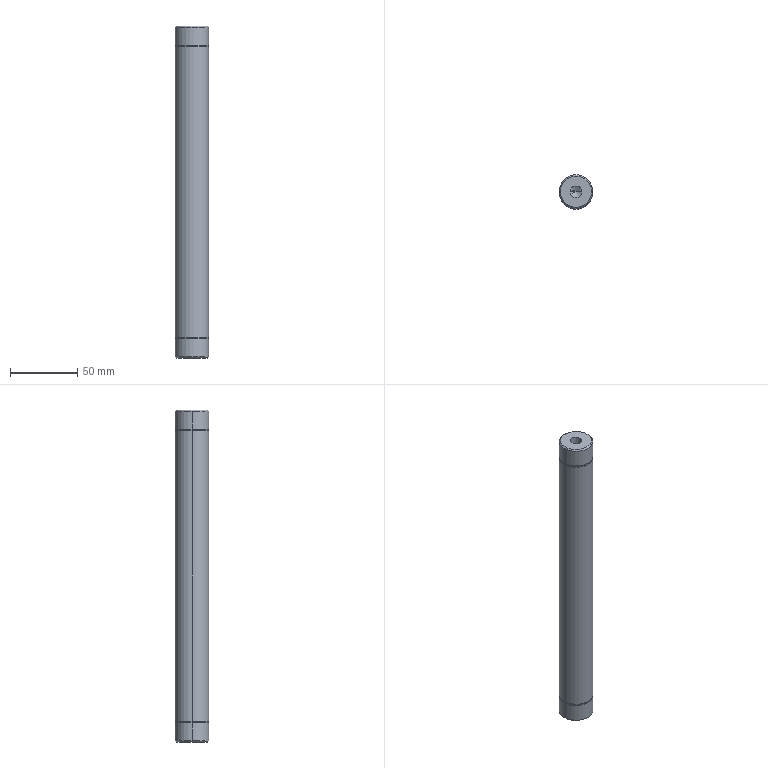Part | STEP file | MM-P46715-03_1 | 1 solid | 28 faces | box 25 x 25 x 246 mm | volume 117700 mm3 | cylinder 14 | cone 8 | plane 6 | commonest cylinder face diameters 25 x6 8.5 x4 23.9 x4